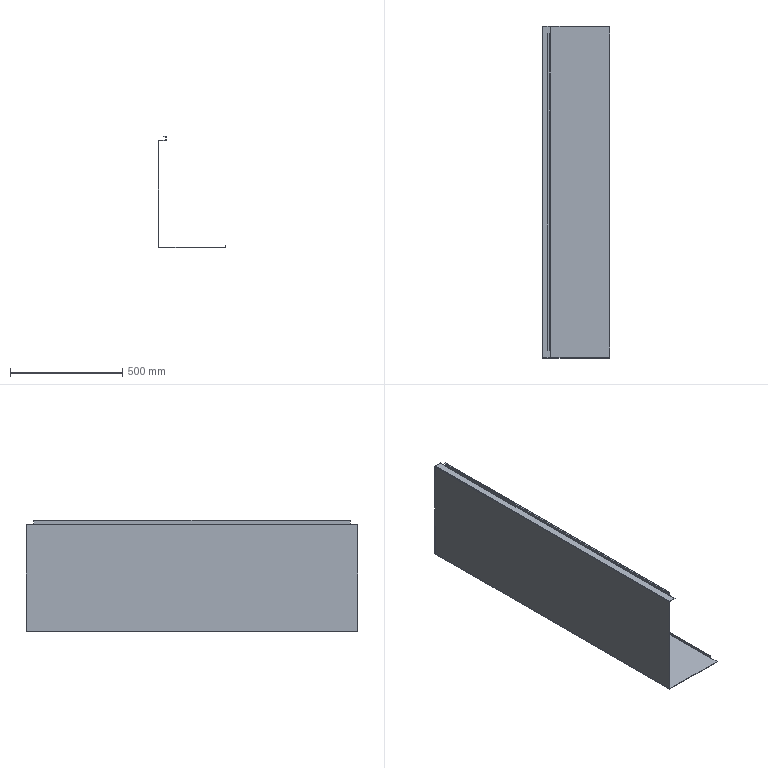Part | SolidWorks | features ICE 3, MoveFace 3, BaseBody 1, Fillet 1 | 1 solid | 52 faces | box 300 x 1476 x 496 mm | volume 2482636 mm3 | plane 36 | cylinder 16 | commonest cylinder face diameters 4.2 x9 0.2 x7